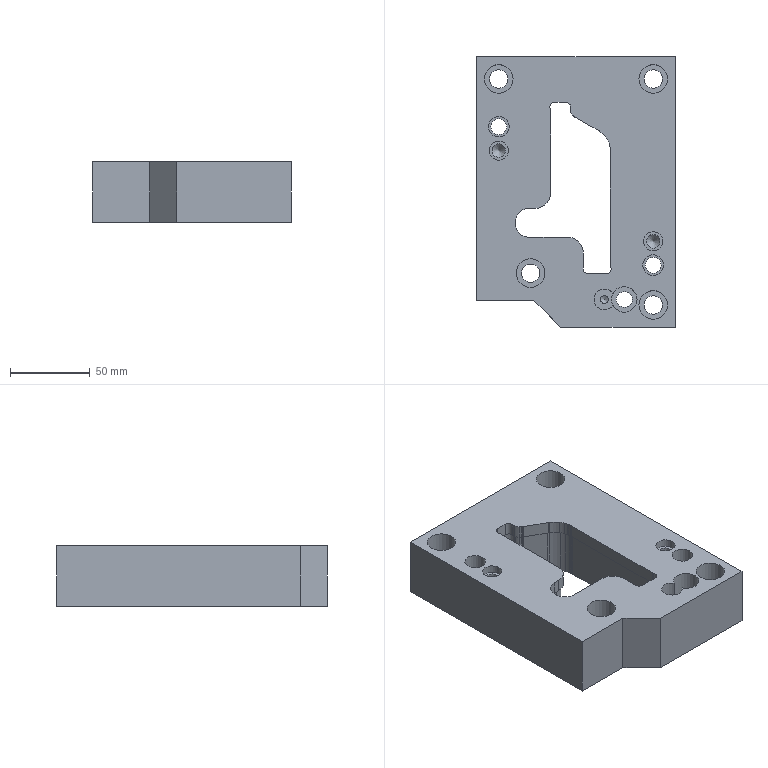Part | STEP file | lll_id150_x_t | 1 solid | 104 faces | box 125 x 170 x 38 mm | volume 581268 mm3 | cylinder 64 | plane 37 | cone 3 | commonest cylinder face diameters 6 x7 9 x4 11.509 x4 17 x4 18.008 x4 20 x4